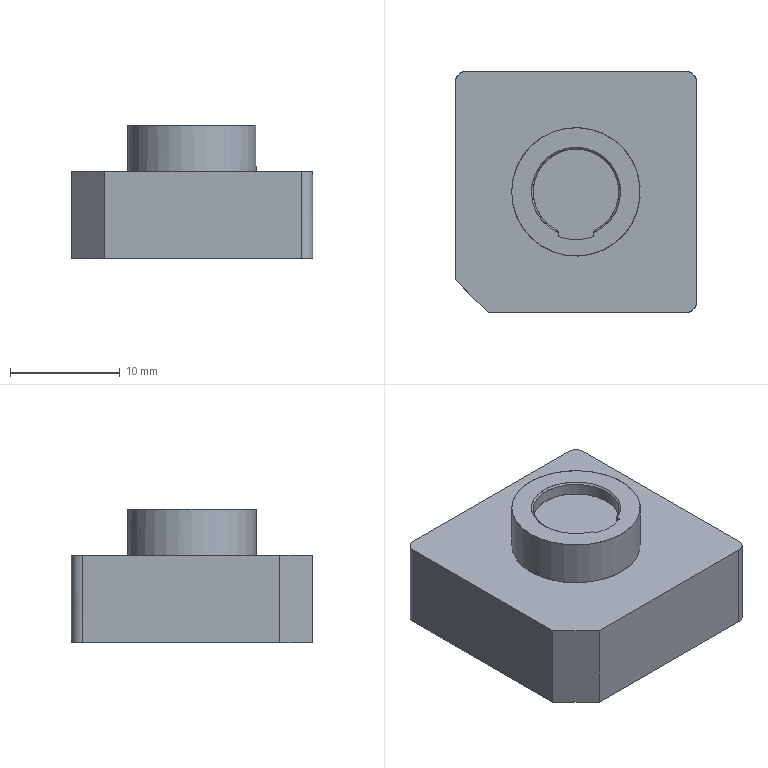NC program | PowerMill | posted by the shop | part box 22 x 22 x 12.219 mm
Lines 2305 to 4803 of 55612, first 2306 of 2499 lines:
( TOOL ID   D3C_1_1 )
( TOOL DIA. 3. TIP RAD 0 LENGTH 59.4 )
( Z = -4.35 )
T15 M6
T3
G91 G28 Z0
G0 G90 G54
M08
S18000 M3
X0 Y0 M8
G43 Z9.799 H15
X-2.901 Y-7.754
Z.842
G1 Z-.358 F3000
X-2.885 Y-7.743 F5000
G3 X-2.84 Y-7.503 I-.098 J.143
G1 X-3.588 Y-6.403
X-4.01 Y-6.167
X-4.647 Y-5.699
X-5.122 Y-5.277
X-5.699 Y-4.647
X-6.167 Y-4.01
X-6.639 Y-3.166
X-6.981 Y-2.322
X-7.206 Y-1.477
X-7.281 Y-1.055
X-7.348 Y-.211
X-7.326 Y.633
X-7.206 Y1.477
X-6.981 Y2.322
X-6.639 Y3.166
X-6.167 Y4.01
X-5.699 Y4.647
X-5.277 Y5.122
X-4.647 Y5.699
X-4.01 Y6.167
X-3.166 Y6.639
X-2.322 Y6.981
X-1.477 Y7.206
X-1.055 Y7.281
X-.211 Y7.348
X.633 Y7.326
X1.477 Y7.206
X2.322 Y6.981
X3.166 Y6.639
X4.01 Y6.167
X4.647 Y5.699
X5.122 Y5.277
X5.699 Y4.647
X6.167 Y4.01
X6.639 Y3.166
X6.981 Y2.322
X7.206 Y1.477
X7.281 Y1.055
X7.348 Y.211
X7.326 Y-.633
X7.206 Y-1.477
X6.981 Y-2.322
X6.639 Y-3.166
X6.167 Y-4.01
X5.699 Y-4.647
X5.277 Y-5.122
X4.647 Y-5.699
X4.01 Y-6.167
X3.166 Y-6.639
X2.367 Y-6.965
X1.477 Y-7.206
X1.055 Y-7.281
X.211 Y-7.348
X-.633 Y-7.326
X-1.477 Y-7.206
X-2.322 Y-6.981
X-3.166 Y-6.639
X-3.588 Y-6.403
X-2.901 Y-7.754 Z-.506
X-2.885 Y-7.743
G3 X-2.84 Y-7.503 I-.098 J.143
G1 X-3.588 Y-6.403
X-4.01 Y-6.167
X-4.647 Y-5.699
X-5.122 Y-5.277
X-5.699 Y-4.647
X-6.167 Y-4.01
X-6.639 Y-3.166
X-6.981 Y-2.322
X-7.206 Y-1.477
X-7.281 Y-1.055
X-7.348 Y-.211
X-7.326 Y.633
X-7.206 Y1.477
X-6.981 Y2.322
X-6.639 Y3.166
X-6.167 Y4.01
X-5.699 Y4.647
X-5.277 Y5.122
X-4.647 Y5.699
X-4.01 Y6.167
X-3.166 Y6.639
X-2.322 Y6.981
X-1.477 Y7.206
X-1.055 Y7.281
X-.211 Y7.348
X.633 Y7.326
X1.477 Y7.206
X2.322 Y6.981
X3.166 Y6.639
X4.01 Y6.167
X4.647 Y5.699
X5.122 Y5.277
X5.699 Y4.647
X6.167 Y4.01
X6.639 Y3.166
X6.981 Y2.322
X7.206 Y1.477
X7.281 Y1.055
X7.348 Y.211
X7.326 Y-.633
X7.206 Y-1.477
X6.981 Y-2.322
X6.639 Y-3.166
X6.167 Y-4.01
X5.699 Y-4.647
X5.277 Y-5.122
X4.647 Y-5.699
X4.01 Y-6.167
X3.166 Y-6.639
X2.367 Y-6.965
X1.477 Y-7.206
X1.055 Y-7.281
X.211 Y-7.348
X-.633 Y-7.326
X-1.477 Y-7.206
X-2.322 Y-6.981
X-3.166 Y-6.639
X-3.588 Y-6.403
X-2.901 Y-7.754 Z-.653
X-2.885 Y-7.743
G3 X-2.84 Y-7.503 I-.098 J.143
G1 X-3.588 Y-6.403
X-4.01 Y-6.167
X-4.647 Y-5.699
X-5.122 Y-5.277
X-5.699 Y-4.647
X-6.167 Y-4.01
X-6.639 Y-3.166
X-6.981 Y-2.322
X-7.206 Y-1.477
X-7.281 Y-1.055
X-7.348 Y-.211
X-7.326 Y.633
X-7.206 Y1.477
X-6.981 Y2.322
X-6.639 Y3.166
X-6.167 Y4.01
X-5.699 Y4.647
X-5.277 Y5.122
X-4.647 Y5.699
X-4.01 Y6.167
X-3.166 Y6.639
X-2.322 Y6.981
X-1.477 Y7.206
X-1.055 Y7.281
X-.211 Y7.348
X.633 Y7.326
X1.477 Y7.206
X2.322 Y6.981
X3.166 Y6.639
X4.01 Y6.167
X4.647 Y5.699
X5.122 Y5.277
X5.699 Y4.647
X6.167 Y4.01
X6.639 Y3.166
X6.981 Y2.322
X7.206 Y1.477
X7.281 Y1.055
X7.348 Y.211
X7.326 Y-.633
X7.206 Y-1.477
X6.981 Y-2.322
X6.639 Y-3.166
X6.167 Y-4.01
X5.699 Y-4.647
X5.277 Y-5.122
X4.647 Y-5.699
X4.01 Y-6.167
X3.166 Y-6.639
X2.367 Y-6.965
X1.477 Y-7.206
X1.055 Y-7.281
X.211 Y-7.348
X-.633 Y-7.326
X-1.477 Y-7.206
X-2.322 Y-6.981
X-3.166 Y-6.639
X-3.588 Y-6.403
X-2.901 Y-7.754 Z-.8
X-2.885 Y-7.743
G3 X-2.84 Y-7.503 I-.098 J.143
G1 X-3.588 Y-6.403
X-4.01 Y-6.167
X-4.647 Y-5.699
X-5.122 Y-5.277
X-5.699 Y-4.647
X-6.167 Y-4.01
X-6.639 Y-3.166
X-6.981 Y-2.322
X-7.206 Y-1.477
X-7.281 Y-1.055
X-7.348 Y-.211
X-7.326 Y.633
X-7.206 Y1.477
X-6.981 Y2.322
X-6.639 Y3.166
X-6.167 Y4.01
X-5.699 Y4.647
X-5.277 Y5.122
X-4.647 Y5.699
X-4.01 Y6.167
X-3.166 Y6.639
X-2.322 Y6.981
X-1.477 Y7.206
X-1.055 Y7.281
X-.211 Y7.348
X.633 Y7.326
X1.477 Y7.206
X2.322 Y6.981
X3.166 Y6.639
X4.01 Y6.167
X4.647 Y5.699
X5.122 Y5.277
X5.699 Y4.647
X6.167 Y4.01
X6.639 Y3.166
X6.981 Y2.322
X7.206 Y1.477
X7.281 Y1.055
X7.348 Y.211
X7.326 Y-.633
X7.206 Y-1.477
X6.981 Y-2.322
X6.639 Y-3.166
X6.167 Y-4.01
X5.699 Y-4.647
X5.277 Y-5.122
X4.647 Y-5.699
X4.01 Y-6.167
X3.166 Y-6.639
X2.367 Y-6.965
X1.477 Y-7.206
X1.055 Y-7.281
X.211 Y-7.348
X-.633 Y-7.326
X-1.477 Y-7.206
X-2.322 Y-6.981
X-3.166 Y-6.639
X-3.588 Y-6.403
X-2.901 Y-7.754 Z-.948
X-2.885 Y-7.743
G3 X-2.84 Y-7.503 I-.098 J.143
G1 X-3.588 Y-6.403
X-4.01 Y-6.167
X-4.647 Y-5.699
X-5.122 Y-5.277
X-5.699 Y-4.647
X-6.167 Y-4.01
X-6.639 Y-3.166
X-6.981 Y-2.322
X-7.206 Y-1.477
X-7.281 Y-1.055
X-7.348 Y-.211
X-7.326 Y.633
X-7.206 Y1.477
X-6.981 Y2.322
X-6.639 Y3.166
X-6.167 Y4.01
X-5.699 Y4.647
X-5.277 Y5.122
X-4.647 Y5.699
X-4.01 Y6.167
X-3.166 Y6.639
X-2.322 Y6.981
X-1.477 Y7.206
X-1.055 Y7.281
X-.211 Y7.348
X.633 Y7.326
X1.477 Y7.206
X2.322 Y6.981
X3.166 Y6.639
X4.01 Y6.167
X4.647 Y5.699
X5.122 Y5.277
X5.699 Y4.647
X6.167 Y4.01
X6.639 Y3.166
X6.981 Y2.322
X7.206 Y1.477
X7.281 Y1.055
X7.348 Y.211
X7.326 Y-.633
X7.206 Y-1.477
X6.981 Y-2.322
X6.639 Y-3.166
X6.167 Y-4.01
X5.699 Y-4.647
X5.277 Y-5.122
X4.647 Y-5.699
X4.01 Y-6.167
X3.166 Y-6.639
X2.367 Y-6.965
X1.477 Y-7.206
X1.055 Y-7.281
X.211 Y-7.348
X-.633 Y-7.326
X-1.477 Y-7.206
X-2.322 Y-6.981
X-3.166 Y-6.639
X-3.588 Y-6.403
X-2.901 Y-7.754 Z-1.095
X-2.885 Y-7.743
G3 X-2.84 Y-7.503 I-.098 J.143
G1 X-3.588 Y-6.403
X-4.01 Y-6.167
X-4.647 Y-5.699
X-5.122 Y-5.277
X-5.699 Y-4.647
X-6.167 Y-4.01
X-6.639 Y-3.166
X-6.981 Y-2.322
X-7.206 Y-1.477
X-7.281 Y-1.055
X-7.348 Y-.211
X-7.326 Y.633
X-7.206 Y1.477
X-6.981 Y2.322
X-6.639 Y3.166
X-6.167 Y4.01
X-5.699 Y4.647
X-5.277 Y5.122
X-4.647 Y5.699
X-4.01 Y6.167
X-3.166 Y6.639
X-2.322 Y6.981
X-1.477 Y7.206
X-1.055 Y7.281
X-.211 Y7.348
X.633 Y7.326
X1.477 Y7.206
X2.322 Y6.981
X3.166 Y6.639
X4.01 Y6.167
X4.647 Y5.699
X5.122 Y5.277
X5.699 Y4.647
X6.167 Y4.01
X6.639 Y3.166
X6.981 Y2.322
X7.206 Y1.477
X7.281 Y1.055
X7.348 Y.211
X7.326 Y-.633
X7.206 Y-1.477
X6.981 Y-2.322
X6.639 Y-3.166
X6.167 Y-4.01
X5.699 Y-4.647
X5.277 Y-5.122
X4.647 Y-5.699
X4.01 Y-6.167
X3.166 Y-6.639
X2.367 Y-6.965
X1.477 Y-7.206
X1.055 Y-7.281
X.211 Y-7.348
X-.633 Y-7.326
X-1.477 Y-7.206
X-2.322 Y-6.981
X-3.166 Y-6.639
X-3.588 Y-6.403
X-2.901 Y-7.754 Z-1.243
X-2.885 Y-7.743
G3 X-2.84 Y-7.503 I-.098 J.143
G1 X-3.588 Y-6.403
X-4.01 Y-6.167
X-4.647 Y-5.699
X-5.122 Y-5.277
X-5.699 Y-4.647
X-6.167 Y-4.01
X-6.639 Y-3.166
X-6.981 Y-2.322
X-7.206 Y-1.477
X-7.281 Y-1.055
X-7.348 Y-.211
X-7.326 Y.633
X-7.206 Y1.477
X-6.981 Y2.322
X-6.639 Y3.166
X-6.167 Y4.01
X-5.699 Y4.647
X-5.277 Y5.122
X-4.647 Y5.699
X-4.01 Y6.167
X-3.166 Y6.639
X-2.322 Y6.981
X-1.477 Y7.206
X-1.055 Y7.281
X-.211 Y7.348
X.633 Y7.326
X1.477 Y7.206
X2.322 Y6.981
X3.166 Y6.639
X4.01 Y6.167
X4.647 Y5.699
X5.122 Y5.277
X5.699 Y4.647
X6.167 Y4.01
X6.639 Y3.166
X6.981 Y2.322
X7.206 Y1.477
X7.281 Y1.055
X7.348 Y.211
X7.326 Y-.633
X7.206 Y-1.477
X6.981 Y-2.322
X6.639 Y-3.166
X6.167 Y-4.01
X5.699 Y-4.647
X5.277 Y-5.122
X4.647 Y-5.699
X4.01 Y-6.167
X3.166 Y-6.639
X2.367 Y-6.965
X1.477 Y-7.206
X1.055 Y-7.281
X.211 Y-7.348
X-.633 Y-7.326
X-1.477 Y-7.206
X-2.322 Y-6.981
X-3.166 Y-6.639
X-3.588 Y-6.403
X-2.901 Y-7.754 Z-1.39
X-2.885 Y-7.743
G3 X-2.84 Y-7.503 I-.098 J.143
G1 X-3.588 Y-6.403
X-4.01 Y-6.167
X-4.647 Y-5.699
X-5.122 Y-5.277
X-5.699 Y-4.647
X-6.167 Y-4.01
X-6.639 Y-3.166
X-6.981 Y-2.322
X-7.206 Y-1.477
X-7.281 Y-1.055
X-7.348 Y-.211
X-7.326 Y.633
X-7.206 Y1.477
X-6.981 Y2.322
X-6.639 Y3.166
X-6.167 Y4.01
X-5.699 Y4.647
X-5.277 Y5.122
X-4.647 Y5.699
X-4.01 Y6.167
X-3.166 Y6.639
X-2.322 Y6.981
X-1.477 Y7.206
X-1.055 Y7.281
X-.211 Y7.348
X.633 Y7.326
X1.477 Y7.206
X2.322 Y6.981
X3.166 Y6.639
X4.01 Y6.167
X4.647 Y5.699
X5.122 Y5.277
X5.699 Y4.647
X6.167 Y4.01
X6.639 Y3.166
X6.981 Y2.322
X7.206 Y1.477
X7.281 Y1.055
X7.348 Y.211
X7.326 Y-.633
X7.206 Y-1.477
X6.981 Y-2.322
X6.639 Y-3.166
X6.167 Y-4.01
X5.699 Y-4.647
X5.277 Y-5.122
X4.647 Y-5.699
X4.01 Y-6.167
X3.166 Y-6.639
X2.367 Y-6.965
X1.477 Y-7.206
X1.055 Y-7.281
X.211 Y-7.348
X-.633 Y-7.326
X-1.477 Y-7.206
X-2.322 Y-6.981
X-3.166 Y-6.639
X-3.588 Y-6.403
X-2.901 Y-7.754 Z-1.538
X-2.885 Y-7.743
G3 X-2.84 Y-7.503 I-.098 J.143
G1 X-3.588 Y-6.403
X-4.01 Y-6.167
X-4.647 Y-5.699
X-5.122 Y-5.277
X-5.699 Y-4.647
X-6.167 Y-4.01
X-6.639 Y-3.166
X-6.981 Y-2.322
X-7.206 Y-1.477
X-7.281 Y-1.055
X-7.348 Y-.211
X-7.326 Y.633
X-7.206 Y1.477
X-6.981 Y2.322
X-6.639 Y3.166
X-6.167 Y4.01
X-5.699 Y4.647
X-5.277 Y5.122
X-4.647 Y5.699
X-4.01 Y6.167
X-3.166 Y6.639
X-2.322 Y6.981
X-1.477 Y7.206
X-1.055 Y7.281
X-.211 Y7.348
X.633 Y7.326
X1.477 Y7.206
X2.322 Y6.981
X3.166 Y6.639
X4.01 Y6.167
X4.647 Y5.699
X5.122 Y5.277
X5.699 Y4.647
X6.167 Y4.01
X6.639 Y3.166
X6.981 Y2.322
X7.206 Y1.477
X7.281 Y1.055
X7.348 Y.211
X7.326 Y-.633
X7.206 Y-1.477
X6.981 Y-2.322
X6.639 Y-3.166
X6.167 Y-4.01
X5.699 Y-4.647
X5.277 Y-5.122
X4.647 Y-5.699
X4.01 Y-6.167
X3.166 Y-6.639
X2.367 Y-6.965
X1.477 Y-7.206
X1.055 Y-7.281
X.211 Y-7.348
X-.633 Y-7.326
X-1.477 Y-7.206
X-2.322 Y-6.981
X-3.166 Y-6.639
X-3.588 Y-6.403
X-2.901 Y-7.754 Z-1.686
X-2.885 Y-7.743
G3 X-2.84 Y-7.503 I-.098 J.143
G1 X-3.588 Y-6.403
X-4.01 Y-6.168
X-4.647 Y-5.699
X-5.122 Y-5.277
X-5.699 Y-4.647
X-6.168 Y-4.01
X-6.639 Y-3.166
X-6.981 Y-2.322
X-7.206 Y-1.477
X-7.281 Y-1.055
X-7.348 Y-.211
X-7.326 Y.633
X-7.206 Y1.477
X-6.981 Y2.322
X-6.639 Y3.166
X-6.168 Y4.01
X-5.699 Y4.647
X-5.277 Y5.122
X-4.647 Y5.699
X-4.01 Y6.168
X-3.166 Y6.639
X-2.322 Y6.981
X-1.477 Y7.206
X-1.055 Y7.281
X-.211 Y7.348
X.633 Y7.326
X1.477 Y7.206
X2.322 Y6.981
X3.166 Y6.639
X4.01 Y6.168
X4.647 Y5.699
X5.122 Y5.277
X5.699 Y4.647
X6.168 Y4.01
X6.639 Y3.166
X6.981 Y2.322
X7.206 Y1.477
X7.281 Y1.055
X7.348 Y.211
X7.326 Y-.633
X7.206 Y-1.477
X6.981 Y-2.322
X6.639 Y-3.166
X6.168 Y-4.01
X5.699 Y-4.647
X5.277 Y-5.122
X4.647 Y-5.699
X4.01 Y-6.168
X3.166 Y-6.639
X2.367 Y-6.965
X1.477 Y-7.206
X1.055 Y-7.281
X.211 Y-7.348
X-.633 Y-7.326
X-1.477 Y-7.206
X-2.322 Y-6.981
X-3.166 Y-6.639
X-3.588 Y-6.403
X-2.901 Y-7.754 Z-1.834
X-2.885 Y-7.743
G3 X-2.84 Y-7.503 I-.098 J.143
G1 X-3.588 Y-6.403
X-4.01 Y-6.168
X-4.647 Y-5.699
X-5.122 Y-5.277
X-5.699 Y-4.647
X-6.168 Y-4.01
X-6.639 Y-3.166
X-6.981 Y-2.322
X-7.206 Y-1.477
X-7.281 Y-1.055
X-7.348 Y-.211
X-7.326 Y.633
X-7.206 Y1.477
X-6.981 Y2.322
X-6.639 Y3.166
X-6.168 Y4.01
X-5.699 Y4.647
X-5.277 Y5.122
X-4.647 Y5.699
X-4.01 Y6.168
X-3.166 Y6.639
X-2.322 Y6.981
X-1.477 Y7.206
X-1.055 Y7.281
X-.211 Y7.348
X.633 Y7.326
X1.477 Y7.206
X2.322 Y6.981
X3.166 Y6.639
X4.01 Y6.168
X4.647 Y5.699
X5.122 Y5.277
X5.699 Y4.647
X6.168 Y4.01
X6.639 Y3.166
X6.981 Y2.322
X7.206 Y1.477
X7.281 Y1.055
X7.348 Y.211
X7.326 Y-.633
X7.206 Y-1.477
X6.981 Y-2.322
X6.639 Y-3.166
X6.168 Y-4.01
X5.699 Y-4.647
X5.277 Y-5.122
X4.647 Y-5.699
X4.01 Y-6.168
X3.166 Y-6.639
X2.367 Y-6.965
X1.477 Y-7.206
X1.055 Y-7.281
X.211 Y-7.348
X-.633 Y-7.326
X-1.477 Y-7.206
X-2.322 Y-6.981
X-3.166 Y-6.639
X-3.588 Y-6.403
X-2.901 Y-7.754 Z-1.982
X-2.885 Y-7.743
G3 X-2.84 Y-7.503 I-.098 J.143
G1 X-3.588 Y-6.403
X-4.01 Y-6.168
X-4.647 Y-5.699
X-5.122 Y-5.277
X-5.699 Y-4.647
X-6.168 Y-4.01
X-6.639 Y-3.166
X-6.981 Y-2.322
X-7.206 Y-1.477
X-7.281 Y-1.055
X-7.348 Y-.211
X-7.326 Y.633
X-7.206 Y1.477
X-6.981 Y2.322
X-6.639 Y3.166
X-6.168 Y4.01
X-5.699 Y4.647
X-5.277 Y5.122
X-4.647 Y5.699
X-4.01 Y6.168
X-3.166 Y6.639
X-2.322 Y6.981
X-1.477 Y7.206
X-1.055 Y7.281
X-.211 Y7.348
X.633 Y7.326
X1.477 Y7.206
X2.322 Y6.981
X3.166 Y6.639
X4.01 Y6.168
X4.647 Y5.699
X5.122 Y5.277
X5.699 Y4.647
X6.168 Y4.01
X6.639 Y3.166
X6.981 Y2.322
X7.206 Y1.477
X7.281 Y1.055
X7.348 Y.211
X7.326 Y-.633
X7.206 Y-1.477
X6.981 Y-2.322
X6.639 Y-3.166
X6.168 Y-4.01
X5.699 Y-4.647
X5.277 Y-5.122
X4.647 Y-5.699
X4.01 Y-6.168
X3.166 Y-6.639
X2.367 Y-6.965
X1.477 Y-7.206
X1.055 Y-7.281
X.211 Y-7.348
X-.633 Y-7.326
X-1.477 Y-7.206
X-2.322 Y-6.981
X-3.166 Y-6.639
X-3.588 Y-6.403
X-2.901 Y-7.754 Z-2.13
X-2.885 Y-7.743
G3 X-2.84 Y-7.503 I-.098 J.143
G1 X-3.588 Y-6.403
X-4.01 Y-6.168
X-4.647 Y-5.699
X-5.122 Y-5.277
X-5.699 Y-4.647
X-6.168 Y-4.01
X-6.639 Y-3.166
X-6.981 Y-2.322
X-7.206 Y-1.477
X-7.281 Y-1.055
X-7.348 Y-.211
X-7.326 Y.633
X-7.206 Y1.477
X-6.981 Y2.322
X-6.639 Y3.166
X-6.168 Y4.01
X-5.699 Y4.647
X-5.277 Y5.122
X-4.647 Y5.699
X-4.01 Y6.168
X-3.166 Y6.639
X-2.322 Y6.981
X-1.477 Y7.206
X-1.055 Y7.281
X-.211 Y7.348
X.633 Y7.326
X1.477 Y7.206
X2.322 Y6.981
X3.166 Y6.639
X4.01 Y6.168
X4.647 Y5.699
X5.122 Y5.277
X5.699 Y4.647
X6.168 Y4.01
X6.639 Y3.166
X6.981 Y2.322
X7.206 Y1.477
X7.281 Y1.055
X7.348 Y.211
X7.326 Y-.633
X7.206 Y-1.477
X6.981 Y-2.322
X6.639 Y-3.166
X6.168 Y-4.01
X5.699 Y-4.647
X5.277 Y-5.122
X4.647 Y-5.699
X4.01 Y-6.168
X3.166 Y-6.639
X2.367 Y-6.965
X1.477 Y-7.206
X1.055 Y-7.281
X.211 Y-7.348
X-.633 Y-7.326
X-1.477 Y-7.206
X-2.322 Y-6.981
X-3.166 Y-6.639
X-3.588 Y-6.403
X-2.901 Y-7.754 Z-2.278
X-2.885 Y-7.743
G3 X-2.84 Y-7.503 I-.098 J.143
G1 X-3.588 Y-6.403
X-4.01 Y-6.168
X-4.647 Y-5.699
X-5.122 Y-5.277
X-5.699 Y-4.647
X-6.168 Y-4.01
X-6.639 Y-3.166
X-6.981 Y-2.322
X-7.206 Y-1.477
X-7.281 Y-1.055
X-7.348 Y-.211
X-7.326 Y.633
X-7.206 Y1.477
X-6.981 Y2.322
X-6.639 Y3.166
X-6.168 Y4.01
X-5.699 Y4.647
X-5.277 Y5.122
X-4.647 Y5.699
X-4.01 Y6.168
X-3.166 Y6.639
X-2.322 Y6.981
X-1.477 Y7.206
X-1.055 Y7.281
X-.211 Y7.348
X.633 Y7.326
X1.477 Y7.206
X2.322 Y6.981
X3.166 Y6.639
X4.01 Y6.168
X4.647 Y5.699
X5.122 Y5.277
X5.699 Y4.647
X6.168 Y4.01
X6.639 Y3.166
X6.981 Y2.322
X7.206 Y1.477
X7.281 Y1.055
X7.348 Y.211
X7.326 Y-.633
X7.206 Y-1.477
X6.981 Y-2.322
X6.639 Y-3.166
X6.168 Y-4.01
X5.699 Y-4.647
X5.277 Y-5.122
X4.647 Y-5.699
X4.01 Y-6.168
X3.166 Y-6.639
X2.367 Y-6.965
X1.477 Y-7.206
X1.055 Y-7.281
X.211 Y-7.348
X-.633 Y-7.326
X-1.477 Y-7.206
X-2.322 Y-6.981
X-3.166 Y-6.639
X-3.588 Y-6.403
X-2.901 Y-7.754 Z-2.426
X-2.885 Y-7.743
G3 X-2.84 Y-7.503 I-.098 J.143
G1 X-3.588 Y-6.403
X-4.01 Y-6.168
X-4.647 Y-5.699
X-5.122 Y-5.277
X-5.699 Y-4.647
X-6.168 Y-4.01
X-6.639 Y-3.166
X-6.981 Y-2.322
X-7.206 Y-1.477
X-7.281 Y-1.055
X-7.348 Y-.211
X-7.326 Y.633
X-7.206 Y1.477
X-6.981 Y2.322
X-6.639 Y3.166
X-6.168 Y4.01
X-5.699 Y4.647
X-5.277 Y5.122
X-4.647 Y5.699
X-4.01 Y6.168
X-3.166 Y6.639
X-2.322 Y6.981
X-1.477 Y7.206
X-1.055 Y7.281
X-.211 Y7.348
X.633 Y7.326
X1.477 Y7.206
X2.322 Y6.981
X3.166 Y6.639
X4.01 Y6.168
X4.647 Y5.699
X5.122 Y5.277
X5.699 Y4.647
X6.168 Y4.01
X6.639 Y3.166
X6.981 Y2.322
X7.206 Y1.477
X7.281 Y1.055
X7.348 Y.211
X7.326 Y-.633
X7.206 Y-1.477
X6.981 Y-2.322
X6.639 Y-3.166
X6.168 Y-4.01
X5.699 Y-4.647
X5.277 Y-5.122
X4.647 Y-5.699
X4.01 Y-6.168
X3.166 Y-6.639
X2.367 Y-6.965
X1.477 Y-7.206
X1.055 Y-7.281
X.211 Y-7.348
X-.633 Y-7.326
X-1.477 Y-7.206
X-2.322 Y-6.981
X-3.166 Y-6.639
X-3.588 Y-6.403
X-2.901 Y-7.754 Z-2.574
X-2.885 Y-7.743
G3 X-2.84 Y-7.503 I-.098 J.143
G1 X-3.588 Y-6.403
X-4.01 Y-6.168
X-4.647 Y-5.699
X-5.122 Y-5.277
X-5.699 Y-4.647
X-6.168 Y-4.01
X-6.639 Y-3.166
X-6.981 Y-2.322
X-7.206 Y-1.477
X-7.281 Y-1.055
X-7.348 Y-.211
X-7.326 Y.633
X-7.206 Y1.477
X-6.981 Y2.322
X-6.639 Y3.166
X-6.168 Y4.01
X-5.699 Y4.647
X-5.277 Y5.122
X-4.647 Y5.699
X-4.01 Y6.168
X-3.166 Y6.639
X-2.322 Y6.981
X-1.477 Y7.206
X-1.055 Y7.281
X-.211 Y7.348
X.633 Y7.326
X1.477 Y7.206
X2.322 Y6.981
X3.166 Y6.639
X4.01 Y6.168
X4.647 Y5.699
X5.122 Y5.277
X5.699 Y4.647
X6.168 Y4.01
X6.639 Y3.166
X6.981 Y2.322
X7.206 Y1.477
X7.281 Y1.055
X7.348 Y.211
X7.326 Y-.633
X7.206 Y-1.477
X6.981 Y-2.322
X6.639 Y-3.166
X6.168 Y-4.01
X5.699 Y-4.647
X5.277 Y-5.122
X4.647 Y-5.699
X4.01 Y-6.168
X3.166 Y-6.639
X2.367 Y-6.965
X1.477 Y-7.206
X1.055 Y-7.281
X.211 Y-7.348
X-.633 Y-7.326
X-1.477 Y-7.206
X-2.322 Y-6.981
X-3.166 Y-6.639
X-3.588 Y-6.403
X-2.901 Y-7.754 Z-2.722
X-2.885 Y-7.743
G3 X-2.84 Y-7.503 I-.098 J.143
G1 X-3.588 Y-6.403
X-4.01 Y-6.168
X-4.647 Y-5.699
X-5.122 Y-5.277
X-5.699 Y-4.647
X-6.168 Y-4.01
X-6.639 Y-3.166
X-6.981 Y-2.322
X-7.206 Y-1.477
X-7.281 Y-1.055
X-7.348 Y-.211
X-7.326 Y.633
X-7.206 Y1.477
X-6.981 Y2.322
X-6.639 Y3.166
X-6.168 Y4.01
X-5.699 Y4.647
X-5.277 Y5.122
X-4.647 Y5.699
X-4.01 Y6.168
X-3.166 Y6.639
X-2.322 Y6.981
X-1.477 Y7.206
X-1.055 Y7.281
X-.211 Y7.348
X.633 Y7.326
X1.477 Y7.206
X2.322 Y6.981
X3.166 Y6.639
X4.01 Y6.168
X4.647 Y5.699
X5.122 Y5.277
X5.699 Y4.647
X6.168 Y4.01
X6.639 Y3.166
X6.981 Y2.322
X7.206 Y1.477
X7.281 Y1.055
X7.348 Y.211
X7.326 Y-.633
X7.206 Y-1.477
X6.981 Y-2.322
X6.639 Y-3.166
X6.168 Y-4.01
X5.699 Y-4.647
X5.277 Y-5.122
X4.647 Y-5.699
X4.01 Y-6.168
X3.166 Y-6.639
X2.367 Y-6.965
X1.477 Y-7.206
X1.055 Y-7.281
X.211 Y-7.348
X-.633 Y-7.326
X-1.477 Y-7.206
X-2.322 Y-6.981
X-3.166 Y-6.639
X-3.588 Y-6.403
X-2.901 Y-7.754 Z-2.87
X-2.885 Y-7.743
G3 X-2.84 Y-7.503 I-.098 J.143
G1 X-3.588 Y-6.403
X-4.01 Y-6.168
X-4.647 Y-5.699
X-5.122 Y-5.277
X-5.699 Y-4.647
X-6.168 Y-4.01
X-6.639 Y-3.166
X-6.981 Y-2.322
X-7.206 Y-1.477
X-7.281 Y-1.055
X-7.348 Y-.211
X-7.326 Y.633
X-7.206 Y1.477
X-6.981 Y2.322
X-6.639 Y3.166
X-6.168 Y4.01
X-5.699 Y4.647
X-5.277 Y5.122
X-4.647 Y5.699
X-4.01 Y6.168
X-3.166 Y6.639
X-2.322 Y6.981
X-1.477 Y7.206
X-1.055 Y7.281
X-.211 Y7.348
X.633 Y7.326
X1.477 Y7.206
X2.322 Y6.981
X3.166 Y6.639
X4.01 Y6.168
X4.647 Y5.699
X5.122 Y5.277
X5.699 Y4.647
X6.168 Y4.01
X6.639 Y3.166
X6.981 Y2.322
X7.206 Y1.477
X7.281 Y1.055
X7.348 Y.211
X7.326 Y-.633
X7.206 Y-1.477
X6.981 Y-2.322
X6.639 Y-3.166
X6.168 Y-4.01
X5.699 Y-4.647
X5.277 Y-5.122
X4.647 Y-5.699
X4.01 Y-6.168
X3.166 Y-6.639
X2.367 Y-6.965
X1.477 Y-7.206
X1.055 Y-7.281
X.211 Y-7.348
X-.633 Y-7.326
X-1.477 Y-7.206
X-2.322 Y-6.981
X-3.166 Y-6.639
X-3.588 Y-6.403
X-2.901 Y-7.754 Z-3.018
X-2.885 Y-7.743
G3 X-2.84 Y-7.503 I-.098 J.143
G1 X-3.588 Y-6.403
X-4.01 Y-6.168
X-4.647 Y-5.699
X-5.122 Y-5.277
X-5.699 Y-4.647
X-6.168 Y-4.01
X-6.639 Y-3.166
X-6.981 Y-2.322
X-7.206 Y-1.477
X-7.281 Y-1.055
X-7.348 Y-.211
X-7.326 Y.633
X-7.206 Y1.477
X-6.981 Y2.322
X-6.639 Y3.166
X-6.168 Y4.01
X-5.699 Y4.647
X-5.277 Y5.122
X-4.647 Y5.699
X-4.01 Y6.168
X-3.166 Y6.639
X-2.322 Y6.981
X-1.477 Y7.206
X-1.055 Y7.281
X-.211 Y7.348
X.633 Y7.326
X1.477 Y7.206
X2.322 Y6.981
X3.166 Y6.639
X4.01 Y6.168
X4.647 Y5.699
X5.122 Y5.277
X5.699 Y4.647
X6.168 Y4.01
X6.639 Y3.166
X6.981 Y2.322
X7.206 Y1.477
X7.281 Y1.055
X7.348 Y.211
X7.326 Y-.633
X7.206 Y-1.477
X6.981 Y-2.322
X6.639 Y-3.166
X6.168 Y-4.01
X5.699 Y-4.647
X5.277 Y-5.122
X4.647 Y-5.699
X4.01 Y-6.168
X3.166 Y-6.639
X2.367 Y-6.965
X1.477 Y-7.206
X1.055 Y-7.281
X.211 Y-7.348
X-.633 Y-7.326
X-1.477 Y-7.206
X-2.322 Y-6.981
X-3.166 Y-6.639
X-3.588 Y-6.403
X-2.901 Y-7.754 Z-3.166
X-2.885 Y-7.743
G3 X-2.84 Y-7.503 I-.098 J.143
G1 X-3.588 Y-6.403
X-4.01 Y-6.168
X-4.647 Y-5.699
X-5.122 Y-5.277
X-5.699 Y-4.647
X-6.168 Y-4.01
X-6.639 Y-3.166
X-6.981 Y-2.322
X-7.206 Y-1.477
X-7.281 Y-1.055
X-7.348 Y-.211
X-7.326 Y.633
X-7.206 Y1.477
X-6.981 Y2.322
X-6.639 Y3.166
X-6.168 Y4.01
X-5.699 Y4.647
X-5.277 Y5.122
X-4.647 Y5.699
X-4.01 Y6.168
X-3.166 Y6.639
X-2.322 Y6.981
X-1.477 Y7.206
X-1.055 Y7.281
X-.211 Y7.348
X.633 Y7.326
X1.477 Y7.206
X2.322 Y6.981
X3.166 Y6.639
X4.01 Y6.168
X4.647 Y5.699
X5.122 Y5.277
X5.699 Y4.647
X6.168 Y4.01
X6.639 Y3.166
X6.981 Y2.322
X7.206 Y1.477
X7.281 Y1.055
X7.348 Y.211
X7.326 Y-.633
X7.206 Y-1.477
X6.981 Y-2.322
X6.639 Y-3.166
X6.168 Y-4.01
X5.699 Y-4.647
X5.277 Y-5.122
X4.647 Y-5.699
X4.01 Y-6.168
X3.166 Y-6.639
X2.367 Y-6.965
X1.477 Y-7.206
X1.055 Y-7.281
X.211 Y-7.348
X-.633 Y-7.326
X-1.477 Y-7.206
X-2.322 Y-6.981
X-3.166 Y-6.639
X-3.588 Y-6.403
X-2.901 Y-7.754 Z-3.314
X-2.885 Y-7.743
G3 X-2.84 Y-7.503 I-.098 J.143
G1 X-3.588 Y-6.403
X-4.01 Y-6.168
X-4.647 Y-5.699
X-5.122 Y-5.277
X-5.699 Y-4.647
X-6.168 Y-4.01
X-6.639 Y-3.166
X-6.981 Y-2.322
X-7.206 Y-1.477
X-7.281 Y-1.055
X-7.348 Y-.211
X-7.326 Y.633
X-7.206 Y1.477
X-6.981 Y2.322
X-6.639 Y3.166
X-6.168 Y4.01
X-5.699 Y4.647
X-5.277 Y5.122
X-4.647 Y5.699
X-4.01 Y6.168
X-3.166 Y6.639
X-2.322 Y6.981
X-1.477 Y7.206
X-1.055 Y7.281
X-.211 Y7.348
X.633 Y7.326
X1.477 Y7.206
X2.322 Y6.981
X3.166 Y6.639
X4.01 Y6.168
X4.647 Y5.699
X5.122 Y5.277
X5.699 Y4.647
X6.168 Y4.01
X6.639 Y3.166
X6.981 Y2.322
X7.206 Y1.477
X7.281 Y1.055
X7.348 Y.211
X7.326 Y-.633
X7.206 Y-1.477
X6.981 Y-2.322
X6.639 Y-3.166
X6.168 Y-4.01
X5.699 Y-4.647
X5.277 Y-5.122
X4.647 Y-5.699
X4.01 Y-6.168
X3.166 Y-6.639
X2.367 Y-6.965
X1.477 Y-7.206
X1.055 Y-7.281
X.211 Y-7.348
X-.633 Y-7.326
X-1.477 Y-7.206
X-2.322 Y-6.981
X-3.166 Y-6.639
X-3.588 Y-6.403
X-2.901 Y-7.754 Z-3.462
X-2.885 Y-7.743
G3 X-2.84 Y-7.503 I-.098 J.143
G1 X-3.588 Y-6.403
X-4.01 Y-6.168
X-4.647 Y-5.699
X-5.122 Y-5.277
X-5.699 Y-4.647
X-6.168 Y-4.01
X-6.639 Y-3.166
X-6.981 Y-2.322
X-7.206 Y-1.477
X-7.281 Y-1.055
X-7.348 Y-.211
X-7.326 Y.633
X-7.206 Y1.477
X-6.981 Y2.322
X-6.639 Y3.166
X-6.168 Y4.01
X-5.699 Y4.647
X-5.277 Y5.122
X-4.647 Y5.699
X-4.01 Y6.168
X-3.166 Y6.639
X-2.322 Y6.981
X-1.477 Y7.206
X-1.055 Y7.281
X-.211 Y7.348
X.633 Y7.326
X1.477 Y7.206
X2.322 Y6.981
X3.166 Y6.639
X4.01 Y6.168
X4.647 Y5.699
X5.122 Y5.277
X5.699 Y4.647
X6.168 Y4.01
X6.639 Y3.166
X6.981 Y2.322
X7.206 Y1.477
X7.281 Y1.055
X7.348 Y.211
X7.326 Y-.633
X7.206 Y-1.477
X6.981 Y-2.322
X6.639 Y-3.166
X6.168 Y-4.01
X5.699 Y-4.647
X5.277 Y-5.122
X4.647 Y-5.699
X4.01 Y-6.168
X3.166 Y-6.639
X2.367 Y-6.965
X1.477 Y-7.206
X1.055 Y-7.281
X.211 Y-7.348
X-.633 Y-7.326
X-1.477 Y-7.206
X-2.322 Y-6.981
X-3.166 Y-6.639
X-3.588 Y-6.403
X-2.901 Y-7.754 Z-3.61
X-2.885 Y-7.743
G3 X-2.84 Y-7.503 I-.098 J.143
G1 X-3.588 Y-6.403
X-4.01 Y-6.168
X-4.647 Y-5.699
X-5.122 Y-5.277
X-5.699 Y-4.647
X-6.168 Y-4.01
X-6.639 Y-3.166
X-6.981 Y-2.322
X-7.206 Y-1.477
X-7.281 Y-1.055
X-7.348 Y-.211
X-7.326 Y.633
X-7.206 Y1.477
X-6.981 Y2.322
X-6.639 Y3.166
X-6.168 Y4.01
X-5.699 Y4.647
X-5.277 Y5.122
X-4.647 Y5.699
X-4.01 Y6.168
X-3.166 Y6.639
X-2.322 Y6.981
X-1.477 Y7.206
X-1.055 Y7.281
X-.211 Y7.348
X.633 Y7.326
X1.477 Y7.206
X2.322 Y6.981
X3.166 Y6.639
X4.01 Y6.168
X4.647 Y5.699
X5.122 Y5.277
X5.699 Y4.647
X6.168 Y4.01
X6.639 Y3.166
X6.981 Y2.322
X7.206 Y1.477
X7.281 Y1.055
X7.348 Y.211
X7.326 Y-.633
X7.206 Y-1.477
X6.981 Y-2.322
X6.639 Y-3.166
X6.168 Y-4.01
X5.699 Y-4.647
X5.277 Y-5.122
X4.647 Y-5.699
X4.01 Y-6.168
X3.166 Y-6.639
X2.367 Y-6.965
X1.477 Y-7.206
X1.055 Y-7.281
X.211 Y-7.348
X-.633 Y-7.326
X-1.477 Y-7.206
X-2.322 Y-6.981
X-3.166 Y-6.639
X-3.588 Y-6.403
X-2.901 Y-7.754 Z-3.758
X-2.885 Y-7.743
G3 X-2.84 Y-7.503 I-.098 J.143
G1 X-3.588 Y-6.403
X-4.01 Y-6.168
X-4.647 Y-5.699
X-5.122 Y-5.277
X-5.699 Y-4.647
X-6.168 Y-4.01
X-6.639 Y-3.166
X-6.981 Y-2.322
X-7.206 Y-1.477
X-7.281 Y-1.055
X-7.348 Y-.211
X-7.326 Y.633
X-7.206 Y1.477
X-6.981 Y2.322
X-6.639 Y3.166
X-6.168 Y4.01
X-5.699 Y4.647
X-5.277 Y5.122
X-4.647 Y5.699
X-4.01 Y6.168
X-3.166 Y6.639
X-2.322 Y6.981
X-1.477 Y7.206
X-1.055 Y7.281
X-.211 Y7.348
X.633 Y7.326
X1.477 Y7.206
X2.322 Y6.981
X3.166 Y6.639
X4.01 Y6.168
X4.647 Y5.699
X5.122 Y5.277
X5.699 Y4.647
X6.168 Y4.01
X6.639 Y3.166
X6.981 Y2.322
X7.206 Y1.477
X7.281 Y1.055
X7.348 Y.211
X7.326 Y-.633
X7.206 Y-1.477
X6.981 Y-2.322
X6.639 Y-3.166
X6.168 Y-4.01
X5.699 Y-4.647
X5.277 Y-5.122
X4.647 Y-5.699
X4.01 Y-6.168
X3.166 Y-6.639
X2.367 Y-6.965
X1.477 Y-7.206
X1.055 Y-7.281
X.211 Y-7.348
X-.633 Y-7.326
X-1.477 Y-7.206
X-2.322 Y-6.981
X-3.166 Y-6.639
X-3.588 Y-6.403
X-2.901 Y-7.754 Z-3.906
X-2.885 Y-7.743
G3 X-2.84 Y-7.503 I-.098 J.143
G1 X-3.588 Y-6.403
X-4.01 Y-6.168
X-4.647 Y-5.699
X-5.122 Y-5.277
X-5.699 Y-4.647
X-6.168 Y-4.01
X-6.639 Y-3.166
X-6.981 Y-2.322
X-7.206 Y-1.477
X-7.281 Y-1.055
X-7.348 Y-.211
X-7.326 Y.633
X-7.206 Y1.477
X-6.981 Y2.322
X-6.639 Y3.166
X-6.168 Y4.01
X-5.699 Y4.647
X-5.277 Y5.122
X-4.647 Y5.699
X-4.01 Y6.168
X-3.166 Y6.639
X-2.322 Y6.981
X-1.477 Y7.206
X-1.055 Y7.281
X-.211 Y7.348
X.633 Y7.326
X1.477 Y7.206
X2.322 Y6.981
X3.166 Y6.639
X4.01 Y6.168
X4.647 Y5.699
X5.122 Y5.277
X5.699 Y4.647
X6.168 Y4.01
X6.639 Y3.166
X6.981 Y2.322
X7.206 Y1.477
X7.281 Y1.055
X7.348 Y.211
X7.326 Y-.633
X7.206 Y-1.477
X6.981 Y-2.322
X6.639 Y-3.166
X6.168 Y-4.01
X5.699 Y-4.647
X5.277 Y-5.122
X4.647 Y-5.699
X4.01 Y-6.168
X3.166 Y-6.639
X2.367 Y-6.965
X1.477 Y-7.206
X1.055 Y-7.281
X.211 Y-7.348
X-.633 Y-7.326
X-1.477 Y-7.206
X-2.322 Y-6.981
X-3.166 Y-6.639
X-3.588 Y-6.403
X-2.901 Y-7.754 Z-4.054
X-2.885 Y-7.743
G3 X-2.84 Y-7.503 I-.098 J.143
G1 X-3.588 Y-6.403
X-4.01 Y-6.168
X-4.647 Y-5.699
X-5.122 Y-5.277
X-5.699 Y-4.647
X-6.168 Y-4.01
X-6.639 Y-3.166
X-6.981 Y-2.322
X-7.206 Y-1.477
X-7.281 Y-1.055
X-7.348 Y-.211
X-7.326 Y.633
X-7.206 Y1.477
X-6.981 Y2.322
X-6.639 Y3.166
X-6.168 Y4.01
X-5.699 Y4.647
X-5.277 Y5.122
X-4.647 Y5.699
X-4.01 Y6.168
X-3.166 Y6.639
X-2.322 Y6.981
X-1.477 Y7.206
X-1.055 Y7.281
X-.211 Y7.348
X.633 Y7.326
X1.477 Y7.206
X2.322 Y6.981
X3.166 Y6.639
X4.01 Y6.168
X4.647 Y5.699
X5.122 Y5.277
X5.699 Y4.647
X6.168 Y4.01
X6.639 Y3.166
X6.981 Y2.322
X7.206 Y1.477
X7.281 Y1.055
X7.348 Y.211
X7.326 Y-.633
X7.206 Y-1.477
X6.981 Y-2.322
X6.639 Y-3.166
X6.168 Y-4.01
X5.699 Y-4.647
X5.277 Y-5.122
X4.647 Y-5.699
X4.01 Y-6.168
X3.166 Y-6.639
X2.367 Y-6.965
X1.477 Y-7.206
X1.055 Y-7.281
X.211 Y-7.348
X-.633 Y-7.326
X-1.477 Y-7.206
X-2.322 Y-6.981
X-3.166 Y-6.639
X-3.588 Y-6.403
X-2.901 Y-7.754 Z-4.202
X-2.885 Y-7.743
G3 X-2.84 Y-7.503 I-.098 J.143
G1 X-3.588 Y-6.403
X-4.01 Y-6.168
X-4.647 Y-5.699
X-5.122 Y-5.277
X-5.699 Y-4.647
X-6.168 Y-4.01
X-6.639 Y-3.166
X-6.981 Y-2.322
X-7.206 Y-1.477
X-7.281 Y-1.055
X-7.348 Y-.211
X-7.326 Y.633
X-7.206 Y1.477
X-6.981 Y2.322
X-6.639 Y3.166
X-6.168 Y4.01
X-5.699 Y4.647
X-5.277 Y5.122
X-4.647 Y5.699
X-4.01 Y6.168
X-3.166 Y6.639
X-2.322 Y6.981
X-1.477 Y7.206
X-1.055 Y7.281
X-.211 Y7.348
X.633 Y7.326
X1.477 Y7.206
X2.322 Y6.981
X3.166 Y6.639
X4.01 Y6.168
X4.647 Y5.699
X5.122 Y5.277
X5.699 Y4.647
X6.168 Y4.01
X6.639 Y3.166
X6.981 Y2.322
X7.206 Y1.477
X7.281 Y1.055
X7.348 Y.211
X7.326 Y-.633
X7.206 Y-1.477
X6.981 Y-2.322
X6.639 Y-3.166
X6.168 Y-4.01
X5.699 Y-4.647
X5.277 Y-5.122
X4.647 Y-5.699
X4.01 Y-6.168
X3.166 Y-6.639
X2.367 Y-6.965
X1.477 Y-7.206
X1.055 Y-7.281
X.211 Y-7.348
X-.633 Y-7.326
X-1.477 Y-7.206
X-2.322 Y-6.981
X-3.166 Y-6.639
X-3.588 Y-6.403
G0 Z2.885
G1 X-13.192 Y-.782 F10000
G0 Z-3.15
G1 Z-4.35 F3000
X-13. Y-.767 F5000
X-7.34 Y-.317
X-7.348 Y-.211
X-7.326 Y.633
X-7.206 Y1.477
X-6.981 Y2.322
X-6.639 Y3.166
X-6.168 Y4.01
X-5.699 Y4.647
X-5.277 Y5.122
X-4.647 Y5.699
X-4.01 Y6.168
X-3.166 Y6.639
X-2.322 Y6.981
X-1.477 Y7.206
X-1.055 Y7.281
X-.211 Y7.348
X.633 Y7.326
X1.477 Y7.206
X2.322 Y6.981
X3.166 Y6.639
X4.01 Y6.168
X4.647 Y5.699
X5.122 Y5.277
X5.699 Y4.647
X6.168 Y4.01
X6.639 Y3.166
X6.981 Y2.322
X7.206 Y1.477
X7.281 Y1.055
X7.348 Y.211
X7.326 Y-.633
X7.206 Y-1.477
X6.981 Y-2.322
X6.639 Y-3.166
X6.168 Y-4.01
X5.699 Y-4.647
X5.277 Y-5.122
X4.647 Y-5.699
X4.01 Y-6.168
X3.166 Y-6.639
X2.367 Y-6.965
X1.477 Y-7.206
X1.055 Y-7.281
X.211 Y-7.348
X-.633 Y-7.326
X-1.477 Y-7.206
X-2.322 Y-6.981
X-3.166 Y-6.639
X-4.01 Y-6.168
X-4.647 Y-5.699
X-5.122 Y-5.277
X-5.184 Y-5.21
X-6.653 Y-6.66
X-7.801 Y-7.791
X-8.111 Y-7.463
X-8.407 Y-7.123
X-8.69 Y-6.783
G3 X-9.395 Y-7.062 I-.307 J-.256
G1 X-9.299 Y-8.738
G3 X-8.737 Y-9.303 I.599 J.034
G1 X-7.09 Y-9.403
G3 X-6.804 Y-8.696 I.024 J.402
G1 X-7.141 Y-8.406
X-7.477 Y-8.106
X-7.801 Y-7.791
X-6.653 Y-6.66
G3 X6.641 Y-6.636 I6.635 J6.544
G1 X7.792 Y-7.763
X8.114 Y-7.42
X8.42 Y-7.063
X8.7 Y-6.723
G2 X9.403 Y-6.998 I.306 J-.252
G1 X9.303 Y-8.738
G2 X8.739 Y-9.303 I-.599 J.035
G1 X7.053 Y-9.403
G2 X6.768 Y-8.696 I-.024 J.402
G1 X7.105 Y-8.406
X7.456 Y-8.092
X7.792 Y-7.763
X6.641 Y-6.636
G3 X9.301 Y-.192 I-6.659 J6.52
X6.52 Y6.526 I-9.319 J.077
G1 X7.65 Y7.674
X7.234 Y8.063
X6.798 Y8.43
X6.454 Y8.704
G2 X6.718 Y9.403 I.245 J.307
G1 X8.733 Y9.303
G2 X9.303 Y8.734 I-.03 J-.599
G1 X9.403 Y6.764
G2 X8.701 Y6.492 I-.396 J-.02
G1 X8.419 Y6.834
X8.046 Y7.264
X7.65 Y7.674
X6.52 Y6.526
G3 X-6.541 Y6.54 I-6.538 J-6.641
G1 X-7.669 Y7.691
X-8.058 Y7.29
X-8.425 Y6.87
X-8.708 Y6.529
G2 X-9.41 Y6.805 I-.306 J.254
G1 X-9.306 Y8.736
G2 X-8.737 Y9.302 I.599 J-.032
G1 X-6.754 Y9.403
G2 X-6.49 Y8.704 I.02 J-.392
G1 X-6.834 Y8.43
X-7.261 Y8.071
X-7.669 Y7.691
X-6.541 Y6.54
G3 X-8.775 Y3.075 I6.523 J-6.656
G1 X-9.192 Y1.928
G2 X-9.65 Y1.543 I-.564 J.205
G1 X-10.328 Y1.422
G2 X-11.034 Y2.013 I-.106 J.591
G1 X-11.017 Y10.418
G2 X-10.417 Y11.017 I.6 J-.001
G1 X10.417
G2 X11.017 Y10.417 I0 J-.6
G1 Y-10.417
G2 X10.417 Y-11.017 I-.6 J0
G1 X-10.417
G2 X-11.017 Y-10.416 I0 J.6
G1 X-11. Y-3.167
G2 X-10.433 Y-2.569 I.6 J-.001
G1 X-9.508 Y-2.519
G2 X-8.908 Y-2.923 I.032 J-.599
G1 X-8.826 Y-3.161
G3 X-6.653 Y-6.66 I8.808 J3.045
G1 X-5.184 Y-5.21
X-5.699 Y-4.647
X-6.168 Y-4.01
X-6.639 Y-3.166
X-6.981 Y-2.322
X-7.206 Y-1.477
X-7.281 Y-1.055
X-7.34 Y-.317
X-13. Y-.767
G0 Z5.782
G1 X-1.687 Y1.658 F10000
G0 Z-.108
G1 X-1.674 Y1.673 Z-.109 F3000
X-1.445 Y1.875 Z-.114
X-1.042 Y2.127 Z-.122
X-.589 Y2.293 Z-.131
X-.209 Y2.357 Z-.137
X.208 Z-.145
X.625 Y2.283 Z-.152
X1.042 Y2.126 Z-.16
X1.096 Y2.092 Z-.161
X1.459 Y1.864 Z-.169
X1.674 Y1.673 Z-.174
X1.875 Y1.444 Z-.179
X2.125 Y1.042 Z-.187
X2.293 Y.604 Z-.195
X2.362 Y.209 Z-.202
X2.359 Y-.208 Z-.21
X2.315 Y-.456 Z-.214
X2.203 Y-.516 Z-.216
X1.668 Y-.678 Z-.226
X1.112 Y-.733 Z-.236
X.556 Y-.678 Z-.245
X.022 Y-.516 Z-.255
X-.471 Y-.253 Z-.265
X-.903 Y.102 Z-.275
X-1.257 Y.534 Z-.284
X-1.521 Y1.026 Z-.294
X-1.683 Y1.561 Z-.304
X-1.692 Y1.653 Z-.306
X-1.674 Y1.673
X-1.445 Y1.875 Z-.311
X-1.042 Y2.127 Z-.32
X-.589 Y2.293 Z-.328
X-.209 Y2.357 Z-.335
X.208 Z-.342
X.625 Y2.283 Z-.349
X1.042 Y2.126 Z-.357
X1.096 Y2.092 Z-.358
X1.112 Y2.117
X.231 Y.464 F5000
G3 X-.365 Y.107 I-.191 J-.358
X.445 Y.107 I.405 J0
X.231 Y.464 I-.405 J0
G1 X1.112 Y2.117
X1.055 Y2.153
X.633 Y2.313
X.211 Y2.387
X-.211
X-.597 Y2.322
X-1.055 Y2.154
X-1.463 Y1.9
X-1.695 Y1.695
X-1.888 Y1.477
X-2.154 Y1.055
X-2.312 Y.633
X-2.392 Y.211
X-2.389 Y-.211
X-2.314 Y-.633
X-2.153 Y-1.055
X-1.887 Y-1.477
X-1.477 Y-1.894
X-.823 Y-2.322
X-.633 Y-2.489
X-.403 Y-2.785
X-.359 Y-2.823
X-.305 Y-2.842
X-.211 Y-2.855
X.211
X.297 Y-2.843
X.357 Y-2.821
X.403 Y-2.776
X.423 Y-2.744
X.633 Y-2.49
X.823 Y-2.322
X1.461 Y-1.9
X1.697 Y-1.697
X1.887 Y-1.477
X2.153 Y-1.055
X2.314 Y-.633
X2.389 Y-.211
X2.392 Y.211
X2.322 Y.612
X2.152 Y1.055
X1.9 Y1.462
X1.695 Y1.695
X1.477 Y1.888
X1.112 Y2.117
X-1.687 Y1.658 Z-.256
X-1.674 Y1.673 F3000
X-1.445 Y1.875 Z-.261
X-1.042 Y2.127 Z-.27
X-.589 Y2.293 Z-.278
X-.209 Y2.357 Z-.285
X.208 Z-.292
X.625 Y2.283 Z-.3
X1.042 Y2.126 Z-.307
X1.096 Y2.092 Z-.308
X1.459 Y1.864 Z-.316
X1.674 Y1.673 Z-.321
X1.875 Y1.444 Z-.326
X2.125 Y1.042 Z-.334
X2.293 Y.604 Z-.343
X2.362 Y.209 Z-.35
X2.359 Y-.208 Z-.357
X2.315 Y-.456 Z-.361
X2.203 Y-.516 Z-.364
X1.668 Y-.678 Z-.373
X1.112 Y-.733 Z-.383
X.556 Y-.678 Z-.393
X.022 Y-.516 Z-.403
X-.471 Y-.253 Z-.412
X-.903 Y.102 Z-.422
X-1.257 Y.534 Z-.432
X-1.521 Y1.026 Z-.442
X-1.683 Y1.561 Z-.451
X-1.692 Y1.653 Z-.453
X-1.674 Y1.673
X-1.445 Y1.875 Z-.459
X-1.042 Y2.127 Z-.467
X-.589 Y2.293 Z-.475
X-.209 Y2.357 Z-.482
X.208 Z-.489
X.625 Y2.283 Z-.497
X1.042 Y2.126 Z-.505
X1.096 Y2.092 Z-.506
X1.112 Y2.117
X.231 Y.464 F5000
G3 X-.365 Y.107 I-.191 J-.358
X.445 Y.107 I.405 J0
X.231 Y.464 I-.405 J0
G1 X1.112 Y2.117
X1.055 Y2.153
X.633 Y2.313
X.211 Y2.387
X-.211
X-.597 Y2.322
X-1.055 Y2.154
X-1.463 Y1.9
X-1.695 Y1.695
X-1.888 Y1.477
X-2.154 Y1.055
X-2.312 Y.633
X-2.392 Y.211
X-2.389 Y-.211
X-2.314 Y-.633
X-2.153 Y-1.055
X-1.887 Y-1.477
X-1.477 Y-1.894
X-.823 Y-2.322
X-.633 Y-2.489
X-.403 Y-2.785
X-.359 Y-2.823
X-.305 Y-2.842
X-.211 Y-2.855
X.211
X.297 Y-2.843
X.357 Y-2.821
X.403 Y-2.776
X.423 Y-2.744
X.633 Y-2.49
X.823 Y-2.322
X1.461 Y-1.9
X1.697 Y-1.697
X1.887 Y-1.477
X2.153 Y-1.055
X2.314 Y-.633
X2.389 Y-.211
X2.392 Y.211
X2.322 Y.612
X2.152 Y1.055
X1.9 Y1.462
X1.695 Y1.695
X1.477 Y1.888
X1.112 Y2.117
X-1.687 Y1.658 Z-.403
X-1.674 Y1.673 F3000
X-1.445 Y1.875 Z-.409
X-1.042 Y2.127 Z-.417
X-.589 Y2.293 Z-.426
X-.209 Y2.357 Z-.432
X.208 Z-.44
X.625 Y2.283 Z-.447
X1.042 Y2.126 Z-.455
X1.096 Y2.092 Z-.456
X1.459 Y1.864 Z-.463
X1.674 Y1.673 Z-.468
X1.875 Y1.444 Z-.474
X2.125 Y1.042 Z-.482
X2.293 Y.604 Z-.49
X2.362 Y.209 Z-.497
X2.359 Y-.208 Z-.504
X2.315 Y-.456 Z-.509
X2.203 Y-.516 Z-.511
X1.668 Y-.678 Z-.521
X1.112 Y-.733 Z-.53
X.556 Y-.678 Z-.54
X.022 Y-.516 Z-.55
X-.471 Y-.253 Z-.56
X-.903 Y.102 Z-.569
X-1.257 Y.534 Z-.579
X-1.521 Y1.026 Z-.589
X-1.683 Y1.561 Z-.599
X-1.692 Y1.653 Z-.6
X-1.674 Y1.673 Z-.601
X-1.445 Y1.875 Z-.606
X-1.042 Y2.127 Z-.614
X-.589 Y2.293 Z-.623
X-.209 Y2.357 Z-.63
X.208 Z-.637
X.625 Y2.283 Z-.644
X1.042 Y2.126 Z-.652
X1.096 Y2.092 Z-.653
X1.112 Y2.117
X.231 Y.464 F5000
G3 X-.365 Y.107 I-.191 J-.358
X.445 Y.107 I.405 J0
X.231 Y.464 I-.405 J0
G1 X1.112 Y2.117
X1.055 Y2.153
X.633 Y2.313
X.211 Y2.387
X-.211
X-.597 Y2.322
X-1.055 Y2.154
X-1.463 Y1.9
X-1.695 Y1.695
X-1.888 Y1.477
X-2.154 Y1.055
X-2.312 Y.633
X-2.392 Y.211
X-2.389 Y-.211
X-2.314 Y-.633
X-2.153 Y-1.055
X-1.887 Y-1.477
X-1.477 Y-1.894
X-.823 Y-2.322
X-.633 Y-2.489
X-.403 Y-2.785
X-.359 Y-2.823
X-.305 Y-2.842
X-.211 Y-2.855
X.211
X.297 Y-2.843
X.357 Y-2.821
X.403 Y-2.776
X.423 Y-2.744
X.633 Y-2.49
X.823 Y-2.322
X1.461 Y-1.9
X1.697 Y-1.697
X1.887 Y-1.477
X2.153 Y-1.055
X2.314 Y-.633
X2.389 Y-.211
X2.392 Y.211
X2.322 Y.612
X2.152 Y1.055
X1.9 Y1.462
X1.695 Y1.695
X1.477 Y1.888
X1.112 Y2.117
X-1.687 Y1.658 Z-.55
X-1.674 Y1.673 Z-.551 F3000
X-1.445 Y1.875 Z-.556
X-1.042 Y2.127 Z-.564
X-.589 Y2.293 Z-.573
X-.209 Y2.357 Z-.58
X.208 Z-.587
X.625 Y2.283 Z-.594
X1.042 Y2.126 Z-.602
X1.096 Y2.092 Z-.603
X1.459 Y1.863 Z-.611
X1.674 Y1.673 Z-.616
X1.875 Y1.444 Z-.621
X2.125 Y1.042 Z-.629
X2.293 Y.604 Z-.637
X2.362 Y.209 Z-.644
X2.359 Y-.208 Z-.652
X2.315 Y-.456 Z-.656
X2.203 Y-.516 Z-.658
X1.668 Y-.678 Z-.668
X1.112 Y-.733 Z-.678
X.556 Y-.678 Z-.688
X.022 Y-.516 Z-.697
X-.471 Y-.253 Z-.707
X-.903 Y.102 Z-.717
X-1.257 Y.534 Z-.727
X-1.521 Y1.026 Z-.736
X-1.683 Y1.561 Z-.746
X-1.692 Y1.653 Z-.748
X-1.674 Y1.673
X-1.445 Y1.875 Z-.753
X-1.042 Y2.127 Z-.762
X-.589 Y2.293 Z-.77
X-.209 Y2.357 Z-.777
X.208 Z-.784
X.625 Y2.283 Z-.792
X1.042 Y2.126 Z-.799
X1.096 Y2.092 Z-.8
X1.112 Y2.117
X.231 Y.464 F5000
G3 X-.365 Y.107 I-.191 J-.358
X.445 Y.107 I.405 J0
X.231 Y.464 I-.405 J0
G1 X1.112 Y2.117
X1.055 Y2.153
X.633 Y2.312
X.211 Y2.387
X-.211
X-.597 Y2.322
X-1.055 Y2.154
X-1.463 Y1.9
X-1.695 Y1.695
X-1.888 Y1.477
X-2.154 Y1.055
X-2.312 Y.633
X-2.392 Y.211
X-2.389 Y-.211
X-2.314 Y-.633
X-2.153 Y-1.055
X-1.887 Y-1.477
X-1.477 Y-1.894
X-.823 Y-2.322
X-.633 Y-2.489
X-.403 Y-2.785
X-.359 Y-2.823
X-.305 Y-2.842
X-.211 Y-2.855
X.211
X.297 Y-2.843
X.357 Y-2.821
X.403 Y-2.776
X.423 Y-2.744
X.633 Y-2.49
X.823 Y-2.322
X1.461 Y-1.9
X1.697 Y-1.697
X1.887 Y-1.477
X2.153 Y-1.055
X2.314 Y-.633
X2.389 Y-.211
X2.392 Y.211
X2.322 Y.612
X2.152 Y1.055
X1.9 Y1.462
X1.695 Y1.695
X1.477 Y1.888
X1.112 Y2.117
X-1.687 Y1.658 Z-.698
X-1.674 Y1.673 F3000
X-1.445 Y1.875 Z-.704
X-1.042 Y2.127 Z-.712
X-.589 Y2.293 Z-.72
X-.209 Y2.357 Z-.727
X.208 Z-.734
X.625 Y2.283 Z-.742
X1.042 Y2.126 Z-.749
X1.096 Y2.092 Z-.751
X1.459 Y1.863 Z-.758
X1.674 Y1.673 Z-.763
X1.875 Y1.444 Z-.768
X2.125 Y1.042 Z-.777
X2.293 Y.604 Z-.785
X2.362 Y.209 Z-.792
X2.359 Y-.208 Z-.799
X2.315 Y-.456 Z-.803
X2.203 Y-.516 Z-.806
X1.668 Y-.678 Z-.815
X1.112 Y-.733 Z-.825
X.556 Y-.678 Z-.835
X.022 Y-.516 Z-.845
X-.471 Y-.253 Z-.854
X-.903 Y.102 Z-.864
X-1.257 Y.534 Z-.874
X-1.521 Y1.026 Z-.884
X-1.683 Y1.561 Z-.893
X-1.692 Y1.653 Z-.895
X-1.674 Y1.673 Z-.896
X-1.445 Y1.875 Z-.901
X-1.042 Y2.127 Z-.909
X-.589 Y2.293 Z-.918
X-.209 Y2.357 Z-.924
X.208 Z-.932
X.625 Y2.283 Z-.939
X1.042 Y2.126 Z-.947
X1.096 Y2.092 Z-.948
X1.112 Y2.117
X.231 Y.464 F5000
G3 X-.365 Y.107 I-.191 J-.358
X.445 Y.107 I.405 J0
X.231 Y.464 I-.405 J0
G1 X1.112 Y2.117
X1.055 Y2.153
X.633 Y2.312
X.211 Y2.387
X-.211
X-.597 Y2.322
X-1.055 Y2.154
X-1.463 Y1.9
X-1.695 Y1.695
X-1.888 Y1.477
X-2.154 Y1.055
X-2.312 Y.633
X-2.392 Y.211
X-2.389 Y-.211
X-2.314 Y-.633
X-2.153 Y-1.055
X-1.887 Y-1.477
X-1.477 Y-1.894
X-.822 Y-2.322
X-.633 Y-2.489
X-.403 Y-2.785
X-.359 Y-2.823
X-.305 Y-2.842
X-.211 Y-2.855
X.211
X.297 Y-2.843
X.357 Y-2.821
X.403 Y-2.776
X.423 Y-2.744
X.633 Y-2.49
X.822 Y-2.322
X1.461 Y-1.9
X1.697 Y-1.697
X1.887 Y-1.477
X2.153 Y-1.055
X2.314 Y-.633
X2.389 Y-.211
X2.392 Y.211
X2.322 Y.612
X2.152 Y1.055
X1.9 Y1.462
X1.695 Y1.695
X1.477 Y1.888
X1.112 Y2.117
X-2.245 Y.726 Z-.845
X-2.127 Y1.042 Z-.851 F3000
X-1.864 Y1.459 Z-.86
X-1.674 Y1.673 Z-.865
X-1.445 Y1.875 Z-.87
X-1.042 Y2.127 Z-.878
X-.589 Y2.293 Z-.887
X-.209 Y2.357 Z-.894
X.04 Z-.898
X.208 Z-.901
X.625 Y2.283 Z-.908
X1.042 Y2.126 Z-.916
X1.459 Y1.863 Z-.925
X1.674 Y1.673 Z-.93
X1.875 Y1.444 Z-.935
X2.125 Y1.042 Z-.943
X2.278 Y.643 Z-.951
X2.055 Y.372 Z-.957
X1.623 Y.018 Z-.966
X1.131 Y-.246 Z-.976
X.596 Y-.408 Z-.986
X.04 Y-.463 Z-.996
X-.516 Y-.408 Z-1.005
X-1.051 Y-.246 Z-1.015
X-1.543 Y.018 Z-1.025
X-1.975 Y.372 Z-1.035
X-2.252 Y.709 Z-1.042
X-2.127 Y1.042 Z-1.049
X-1.864 Y1.459 Z-1.057
X-1.674 Y1.673 Z-1.062
X-1.445 Y1.875 Z-1.067
X-1.042 Y2.127 Z-1.076
X-.589 Y2.293 Z-1.084
X-.209 Y2.357 Z-1.091
X.04 Z-1.095
Y2.387
Y.512 F5000
G3 X-.365 Y.107 I0 J-.405
X.445 Y.107 I.405 J0
X.04 Y.512 I-.405 J0
G1 Y2.387
X-.211
X-.597 Y2.322
X-1.055 Y2.154
X-1.463 Y1.9
X-1.695 Y1.695
X-1.888 Y1.477
X-2.154 Y1.055
X-2.312 Y.633
X-2.392 Y.211
X-2.389 Y-.211
X-2.314 Y-.633
X-2.153 Y-1.055
X-1.887 Y-1.477
X-1.477 Y-1.894
X-.822 Y-2.322
X-.633 Y-2.489
X-.403 Y-2.785
X-.359 Y-2.823
X-.305 Y-2.842
X-.211 Y-2.855
X.211
X.297 Y-2.843
X.357 Y-2.821
X.403 Y-2.776
X.423 Y-2.744
X.633 Y-2.489